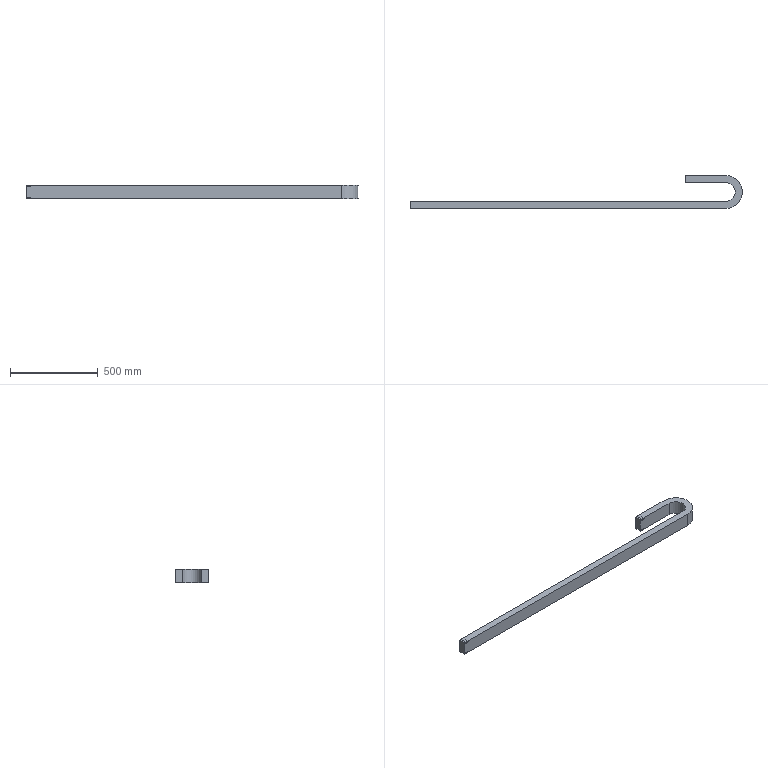Part | SolidWorks | features HoleWzd 2, Extrusion 1 | 1 solid | 26 faces | box 1895 x 190 x 79 mm | volume 7147042 mm3 | cylinder 18 | plane 8 | commonest cylinder face diameters 7 x16 110 x1 190 x1
STEP:
#1=CARTESIAN_POINT('',(-317.901,19.409,1.5));
#2=VERTEX_POINT('',#1);
#3=CARTESIAN_POINT('',(-317.901,19.409,8.5));
#4=VERTEX_POINT('',#3);
#5=CARTESIAN_POINT('',(-317.901,19.409,5.));
#6=DIRECTION('',(0.,1.,0.));
#7=DIRECTION('',(0.,0.,1.));
#8=AXIS2_PLACEMENT_3D('',#5,#6,#7);
#9=CIRCLE('',#8,3.5);
#10=EDGE_CURVE('',#2,#4,#9,.T.);
#11=ORIENTED_EDGE('',*,*,#10,.F.);
#12=CARTESIAN_POINT('',(-317.901,59.409,1.5));
#13=VERTEX_POINT('',#12);
#14=CARTESIAN_POINT('',(-317.901,59.409,1.5));
#15=DIRECTION('',(0.,1.,0.));
#16=VECTOR('',#15,1000.);
#17=LINE('',#14,#16);
#18=EDGE_CURVE('',#2,#13,#17,.T.);
#19=ORIENTED_EDGE('',*,*,#18,.T.);
#20=CARTESIAN_POINT('',(-317.901,59.409,8.5));
#21=VERTEX_POINT('',#20);
#22=CARTESIAN_POINT('',(-317.901,59.409,5.));
#23=DIRECTION('',(0.,1.,0.));
#24=DIRECTION('',(0.,0.,1.));
#25=AXIS2_PLACEMENT_3D('',#22,#23,#24);
#26=CIRCLE('',#25,3.5);
#27=EDGE_CURVE('',#13,#21,#26,.T.);
#28=ORIENTED_EDGE('',*,*,#27,.T.);
#29=CARTESIAN_POINT('',(-317.901,59.409,8.5));
#30=DIRECTION('',(0.,1.,0.));
#31=VECTOR('',#30,1000.);
#32=LINE('',#29,#31);
#33=EDGE_CURVE('',#4,#21,#32,.T.);
#34=ORIENTED_EDGE('',*,*,#33,.F.);
#35=EDGE_LOOP('',(#11,#19,#28,#34));
#36=FACE_OUTER_BOUND('',#35,.T.);
#37=CARTESIAN_POINT('',(-317.901,59.409,5.));
#38=DIRECTION('',(0.,1.,0.));
#39=DIRECTION('',(0.,0.,1.));
#40=AXIS2_PLACEMENT_3D('',#37,#38,#39);
#41=CYLINDRICAL_SURFACE('',#40,3.5);
#42=ADVANCED_FACE('',(#36),#41,.F.);
#43=CARTESIAN_POINT('',(-302.901,19.409,1.5));
#44=VERTEX_POINT('',#43);
#45=CARTESIAN_POINT('',(-302.901,19.409,8.5));
#46=VERTEX_POINT('',#45);
#47=CARTESIAN_POINT('',(-302.901,19.409,5.));
#48=DIRECTION('',(0.,1.,0.));
#49=DIRECTION('',(0.,0.,1.));
#50=AXIS2_PLACEMENT_3D('',#47,#48,#49);
#51=CIRCLE('',#50,3.5);
#52=EDGE_CURVE('',#44,#46,#51,.T.);
#53=ORIENTED_EDGE('',*,*,#52,.F.);
#54=CARTESIAN_POINT('',(-302.901,59.409,1.5));
#55=VERTEX_POINT('',#54);
#56=CARTESIAN_POINT('',(-302.901,59.409,1.5));
#57=DIRECTION('',(0.,1.,0.));
#58=VECTOR('',#57,1000.);
#59=LINE('',#56,#58);
#60=EDGE_CURVE('',#44,#55,#59,.T.);
#61=ORIENTED_EDGE('',*,*,#60,.T.);
#62=CARTESIAN_POINT('',(-302.901,59.409,8.5));
#63=VERTEX_POINT('',#62);
#64=CARTESIAN_POINT('',(-302.901,59.409,5.));
#65=DIRECTION('',(0.,1.,0.));
#66=DIRECTION('',(0.,0.,1.));
#67=AXIS2_PLACEMENT_3D('',#64,#65,#66);
#68=CIRCLE('',#67,3.5);
#69=EDGE_CURVE('',#55,#63,#68,.T.);
#70=ORIENTED_EDGE('',*,*,#69,.T.);
#71=CARTESIAN_POINT('',(-302.901,59.409,8.5));
#72=DIRECTION('',(0.,1.,0.));
#73=VECTOR('',#72,1000.);
#74=LINE('',#71,#73);
#75=EDGE_CURVE('',#46,#63,#74,.T.);
#76=ORIENTED_EDGE('',*,*,#75,.F.);
#77=EDGE_LOOP('',(#53,#61,#70,#76));
#78=FACE_OUTER_BOUND('',#77,.T.);
#79=CARTESIAN_POINT('',(-302.901,59.409,5.));
#80=DIRECTION('',(0.,1.,0.));
#81=DIRECTION('',(0.,0.,1.));
#82=AXIS2_PLACEMENT_3D('',#79,#80,#81);
#83=CYLINDRICAL_SURFACE('',#82,3.5);
#84=ADVANCED_FACE('',(#78),#83,.F.);
#85=CARTESIAN_POINT('',(-317.901,19.409,70.5));
#86=VERTEX_POINT('',#85);
#87=CARTESIAN_POINT('',(-317.901,19.409,77.5));
#88=VERTEX_POINT('',#87);
#89=CARTESIAN_POINT('',(-317.901,19.409,74.));
#90=DIRECTION('',(0.,1.,0.));
#91=DIRECTION('',(0.,0.,1.));
#92=AXIS2_PLACEMENT_3D('',#89,#90,#91);
#93=CIRCLE('',#92,3.5);
#94=EDGE_CURVE('',#86,#88,#93,.T.);
#95=ORIENTED_EDGE('',*,*,#94,.F.);
#96=CARTESIAN_POINT('',(-317.901,59.409,70.5));
#97=VERTEX_POINT('',#96);
#98=CARTESIAN_POINT('',(-317.901,59.409,70.5));
#99=DIRECTION('',(0.,1.,0.));
#100=VECTOR('',#99,1000.);
#101=LINE('',#98,#100);
#102=EDGE_CURVE('',#86,#97,#101,.T.);
#103=ORIENTED_EDGE('',*,*,#102,.T.);
#104=CARTESIAN_POINT('',(-317.901,59.409,77.5));
#105=VERTEX_POINT('',#104);
#106=CARTESIAN_POINT('',(-317.901,59.409,74.));
#107=DIRECTION('',(0.,1.,0.));
#108=DIRECTION('',(0.,0.,1.));
#109=AXIS2_PLACEMENT_3D('',#106,#107,#108);
#110=CIRCLE('',#109,3.5);
#111=EDGE_CURVE('',#97,#105,#110,.T.);
#112=ORIENTED_EDGE('',*,*,#111,.T.);
#113=CARTESIAN_POINT('',(-317.901,59.409,77.5));
#114=DIRECTION('',(0.,1.,0.));
#115=VECTOR('',#114,1000.);
#116=LINE('',#113,#115);
#117=EDGE_CURVE('',#88,#105,#116,.T.);
#118=ORIENTED_EDGE('',*,*,#117,.F.);
#119=EDGE_LOOP('',(#95,#103,#112,#118));
#120=FACE_OUTER_BOUND('',#119,.T.);
#121=CARTESIAN_POINT('',(-317.901,59.409,74.));
#122=DIRECTION('',(0.,1.,0.));
#123=DIRECTION('',(0.,0.,1.));
#124=AXIS2_PLACEMENT_3D('',#121,#122,#123);
#125=CYLINDRICAL_SURFACE('',#124,3.5);
#126=ADVANCED_FACE('',(#120),#125,.F.);
#127=CARTESIAN_POINT('',(-302.901,19.409,70.5));
#128=VERTEX_POINT('',#127);
#129=CARTESIAN_POINT('',(-302.901,19.409,77.5));
#130=VERTEX_POINT('',#129);
#131=CARTESIAN_POINT('',(-302.901,19.409,74.));
#132=DIRECTION('',(0.,1.,0.));
#133=DIRECTION('',(0.,0.,1.));
#134=AXIS2_PLACEMENT_3D('',#131,#132,#133);
#135=CIRCLE('',#134,3.5);
#136=EDGE_CURVE('',#128,#130,#135,.T.);
#137=ORIENTED_EDGE('',*,*,#136,.F.);
#138=CARTESIAN_POINT('',(-302.901,59.409,70.5));
#139=VERTEX_POINT('',#138);
#140=CARTESIAN_POINT('',(-302.901,59.409,70.5));
#141=DIRECTION('',(0.,1.,0.));
#142=VECTOR('',#141,1000.);
#143=LINE('',#140,#142);
#144=EDGE_CURVE('',#128,#139,#143,.T.);
#145=ORIENTED_EDGE('',*,*,#144,.T.);
#146=CARTESIAN_POINT('',(-302.901,59.409,77.5));
#147=VERTEX_POINT('',#146);
#148=CARTESIAN_POINT('',(-302.901,59.409,74.));
#149=DIRECTION('',(0.,1.,0.));
#150=DIRECTION('',(0.,0.,1.));
#151=AXIS2_PLACEMENT_3D('',#148,#149,#150);
#152=CIRCLE('',#151,3.5);
#153=EDGE_CURVE('',#139,#147,#152,.T.);
#154=ORIENTED_EDGE('',*,*,#153,.T.);
#155=CARTESIAN_POINT('',(-302.901,59.409,77.5));
#156=DIRECTION('',(0.,1.,0.));
#157=VECTOR('',#156,1000.);
#158=LINE('',#155,#157);
#159=EDGE_CURVE('',#130,#147,#158,.T.);
#160=ORIENTED_EDGE('',*,*,#159,.F.);
#161=EDGE_LOOP('',(#137,#145,#154,#160));
#162=FACE_OUTER_BOUND('',#161,.T.);
#163=CARTESIAN_POINT('',(-302.901,59.409,74.));
#164=DIRECTION('',(0.,1.,0.));
#165=DIRECTION('',(0.,0.,1.));
#166=AXIS2_PLACEMENT_3D('',#163,#164,#165);
#167=CYLINDRICAL_SURFACE('',#166,3.5);
#168=ADVANCED_FACE('',(#162),#167,.F.);
#169=CARTESIAN_POINT('',(-1872.901,-90.591,8.5));
#170=VERTEX_POINT('',#169);
#171=CARTESIAN_POINT('',(-1872.901,-90.591,1.5));
#172=VERTEX_POINT('',#171);
#173=CARTESIAN_POINT('',(-1872.901,-90.591,5.));
#174=DIRECTION('',(0.,-1.,0.));
#175=DIRECTION('',(1.,0.,0.));
#176=AXIS2_PLACEMENT_3D('',#173,#174,#175);
#177=CIRCLE('',#176,3.5);
#178=EDGE_CURVE('',#170,#172,#177,.T.);
#179=ORIENTED_EDGE('',*,*,#178,.F.);
#180=CARTESIAN_POINT('',(-1872.901,-130.591,8.5));
#181=VERTEX_POINT('',#180);
#182=CARTESIAN_POINT('',(-1872.901,-130.591,8.5));
#183=DIRECTION('',(0.,-1.,0.));
#184=VECTOR('',#183,1000.);
#185=LINE('',#182,#184);
#186=EDGE_CURVE('',#170,#181,#185,.T.);
#187=ORIENTED_EDGE('',*,*,#186,.T.);
#188=CARTESIAN_POINT('',(-1872.901,-130.591,1.5));
#189=VERTEX_POINT('',#188);
#190=CARTESIAN_POINT('',(-1872.901,-130.591,5.));
#191=DIRECTION('',(0.,-1.,0.));
#192=DIRECTION('',(0.,0.,-1.));
#193=AXIS2_PLACEMENT_3D('',#190,#191,#192);
#194=CIRCLE('',#193,3.5);
#195=EDGE_CURVE('',#181,#189,#194,.T.);
#196=ORIENTED_EDGE('',*,*,#195,.T.);
#197=CARTESIAN_POINT('',(-1872.901,-130.591,1.5));
#198=DIRECTION('',(0.,-1.,0.));
#199=VECTOR('',#198,1000.);
#200=LINE('',#197,#199);
#201=EDGE_CURVE('',#172,#189,#200,.T.);
#202=ORIENTED_EDGE('',*,*,#201,.F.);
#203=EDGE_LOOP('',(#179,#187,#196,#202));
#204=FACE_OUTER_BOUND('',#203,.T.);
#205=CARTESIAN_POINT('',(-1872.901,-130.591,5.));
#206=DIRECTION('',(0.,-1.,0.));
#207=DIRECTION('',(0.,0.,-1.));
#208=AXIS2_PLACEMENT_3D('',#205,#206,#207);
#209=CYLINDRICAL_SURFACE('',#208,3.5);
#210=ADVANCED_FACE('',(#204),#209,.F.);
#211=CARTESIAN_POINT('',(-1887.901,-90.591,8.5));
#212=VERTEX_POINT('',#211);
#213=CARTESIAN_POINT('',(-1887.901,-90.591,1.5));
#214=VERTEX_POINT('',#213);
#215=CARTESIAN_POINT('',(-1887.901,-90.591,5.));
#216=DIRECTION('',(0.,-1.,0.));
#217=DIRECTION('',(1.,0.,0.));
#218=AXIS2_PLACEMENT_3D('',#215,#216,#217);
#219=CIRCLE('',#218,3.5);
#220=EDGE_CURVE('',#212,#214,#219,.T.);
#221=ORIENTED_EDGE('',*,*,#220,.F.);
#222=CARTESIAN_POINT('',(-1887.901,-130.591,8.5));
#223=VERTEX_POINT('',#222);
#224=CARTESIAN_POINT('',(-1887.901,-130.591,8.5));
#225=DIRECTION('',(0.,-1.,0.));
#226=VECTOR('',#225,1000.);
#227=LINE('',#224,#226);
#228=EDGE_CURVE('',#212,#223,#227,.T.);
#229=ORIENTED_EDGE('',*,*,#228,.T.);
#230=CARTESIAN_POINT('',(-1887.901,-130.591,1.5));
#231=VERTEX_POINT('',#230);
#232=CARTESIAN_POINT('',(-1887.901,-130.591,5.));
#233=DIRECTION('',(0.,-1.,0.));
#234=DIRECTION('',(0.,0.,-1.));
#235=AXIS2_PLACEMENT_3D('',#232,#233,#234);
#236=CIRCLE('',#235,3.5);
#237=EDGE_CURVE('',#223,#231,#236,.T.);
#238=ORIENTED_EDGE('',*,*,#237,.T.);
#239=CARTESIAN_POINT('',(-1887.901,-130.591,1.5));
#240=DIRECTION('',(0.,-1.,0.));
#241=VECTOR('',#240,1000.);
#242=LINE('',#239,#241);
#243=EDGE_CURVE('',#214,#231,#242,.T.);
#244=ORIENTED_EDGE('',*,*,#243,.F.);
#245=EDGE_LOOP('',(#221,#229,#238,#244));
#246=FACE_OUTER_BOUND('',#245,.T.);
#247=CARTESIAN_POINT('',(-1887.901,-130.591,5.));
#248=DIRECTION('',(0.,-1.,0.));
#249=DIRECTION('',(0.,0.,-1.));
#250=AXIS2_PLACEMENT_3D('',#247,#248,#249);
#251=CYLINDRICAL_SURFACE('',#250,3.5);
#252=ADVANCED_FACE('',(#246),#251,.F.);
#253=CARTESIAN_POINT('',(-1872.901,-90.591,77.5));
#254=VERTEX_POINT('',#253);
#255=CARTESIAN_POINT('',(-1872.901,-90.591,70.5));
#256=VERTEX_POINT('',#255);
#257=CARTESIAN_POINT('',(-1872.901,-90.591,74.));
#258=DIRECTION('',(0.,-1.,0.));
#259=DIRECTION('',(1.,0.,0.));
#260=AXIS2_PLACEMENT_3D('',#257,#258,#259);
#261=CIRCLE('',#260,3.5);
#262=EDGE_CURVE('',#254,#256,#261,.T.);
#263=ORIENTED_EDGE('',*,*,#262,.F.);
#264=CARTESIAN_POINT('',(-1872.901,-130.591,77.5));
#265=VERTEX_POINT('',#264);
#266=CARTESIAN_POINT('',(-1872.901,-130.591,77.5));
#267=DIRECTION('',(0.,-1.,0.));
#268=VECTOR('',#267,1000.);
#269=LINE('',#266,#268);
#270=EDGE_CURVE('',#254,#265,#269,.T.);
#271=ORIENTED_EDGE('',*,*,#270,.T.);
#272=CARTESIAN_POINT('',(-1872.901,-130.591,70.5));
#273=VERTEX_POINT('',#272);
#274=CARTESIAN_POINT('',(-1872.901,-130.591,74.));
#275=DIRECTION('',(0.,-1.,0.));
#276=DIRECTION('',(0.,0.,-1.));
#277=AXIS2_PLACEMENT_3D('',#274,#275,#276);
#278=CIRCLE('',#277,3.5);
#279=EDGE_CURVE('',#265,#273,#278,.T.);
#280=ORIENTED_EDGE('',*,*,#279,.T.);
#281=CARTESIAN_POINT('',(-1872.901,-130.591,70.5));
#282=DIRECTION('',(0.,-1.,0.));
#283=VECTOR('',#282,1000.);
#284=LINE('',#281,#283);
#285=EDGE_CURVE('',#256,#273,#284,.T.);
#286=ORIENTED_EDGE('',*,*,#285,.F.);
#287=EDGE_LOOP('',(#263,#271,#280,#286));
#288=FACE_OUTER_BOUND('',#287,.T.);
#289=CARTESIAN_POINT('',(-1872.901,-130.591,74.));
#290=DIRECTION('',(0.,-1.,0.));
#291=DIRECTION('',(0.,0.,-1.));
#292=AXIS2_PLACEMENT_3D('',#289,#290,#291);
#293=CYLINDRICAL_SURFACE('',#292,3.5);
#294=ADVANCED_FACE('',(#288),#293,.F.);
#295=CARTESIAN_POINT('',(-1887.901,-90.591,77.5));
#296=VERTEX_POINT('',#295);
#297=CARTESIAN_POINT('',(-1887.901,-90.591,70.5));
#298=VERTEX_POINT('',#297);
#299=CARTESIAN_POINT('',(-1887.901,-90.591,74.));
#300=DIRECTION('',(0.,-1.,0.));
#301=DIRECTION('',(1.,0.,0.));
#302=AXIS2_PLACEMENT_3D('',#299,#300,#301);
#303=CIRCLE('',#302,3.5);
#304=EDGE_CURVE('',#296,#298,#303,.T.);
#305=ORIENTED_EDGE('',*,*,#304,.F.);
#306=CARTESIAN_POINT('',(-1887.901,-130.591,77.5));
#307=VERTEX_POINT('',#306);
#308=CARTESIAN_POINT('',(-1887.901,-130.591,77.5));
#309=DIRECTION('',(0.,-1.,0.));
#310=VECTOR('',#309,1000.);
#311=LINE('',#308,#310);
#312=EDGE_CURVE('',#296,#307,#311,.T.);
#313=ORIENTED_EDGE('',*,*,#312,.T.);
#314=CARTESIAN_POINT('',(-1887.901,-130.591,70.5));
#315=VERTEX_POINT('',#314);
#316=CARTESIAN_POINT('',(-1887.901,-130.591,74.));
#317=DIRECTION('',(0.,-1.,0.));
#318=DIRECTION('',(0.,0.,-1.));
#319=AXIS2_PLACEMENT_3D('',#316,#317,#318);
#320=CIRCLE('',#319,3.5);
#321=EDGE_CURVE('',#307,#315,#320,.T.);
#322=ORIENTED_EDGE('',*,*,#321,.T.);
#323=CARTESIAN_POINT('',(-1887.901,-130.591,70.5));
#324=DIRECTION('',(0.,-1.,0.));
#325=VECTOR('',#324,1000.);
#326=LINE('',#323,#325);
#327=EDGE_CURVE('',#298,#315,#326,.T.);
#328=ORIENTED_EDGE('',*,*,#327,.F.);
#329=EDGE_LOOP('',(#305,#313,#322,#328));
#330=FACE_OUTER_BOUND('',#329,.T.);
#331=CARTESIAN_POINT('',(-1887.901,-130.591,74.));
#332=DIRECTION('',(0.,-1.,0.));
#333=DIRECTION('',(0.,0.,-1.));
#334=AXIS2_PLACEMENT_3D('',#331,#332,#333);
#335=CYLINDRICAL_SURFACE('',#334,3.5);
#336=ADVANCED_FACE('',(#330),#335,.F.);
#337=CARTESIAN_POINT('',(-1872.901,-130.591,5.));
#338=DIRECTION('',(0.,-1.,0.));
#339=DIRECTION('',(0.,0.,-1.));
#340=AXIS2_PLACEMENT_3D('',#337,#338,#339);
#341=CIRCLE('',#340,3.5);
#342=EDGE_CURVE('',#189,#181,#341,.T.);
#343=ORIENTED_EDGE('',*,*,#342,.F.);
#344=ORIENTED_EDGE('',*,*,#195,.F.);
#345=EDGE_LOOP('',(#343,#344));
#346=FACE_BOUND('',#345,.T.);
#347=CARTESIAN_POINT('',(-1887.901,-130.591,5.));
#348=DIRECTION('',(0.,-1.,0.));
#349=DIRECTION('',(0.,0.,-1.));
#350=AXIS2_PLACEMENT_3D('',#347,#348,#349);
#351=CIRCLE('',#350,3.5);
#352=EDGE_CURVE('',#231,#223,#351,.T.);
#353=ORIENTED_EDGE('',*,*,#352,.F.);
#354=ORIENTED_EDGE('',*,*,#237,.F.);
#355=EDGE_LOOP('',(#353,#354));
#356=FACE_BOUND('',#355,.T.);
#357=CARTESIAN_POINT('',(-1872.901,-130.591,74.));
#358=DIRECTION('',(0.,-1.,0.));
#359=DIRECTION('',(0.,0.,-1.));
#360=AXIS2_PLACEMENT_3D('',#357,#358,#359);
#361=CIRCLE('',#360,3.5);
#362=EDGE_CURVE('',#273,#265,#361,.T.);
#363=ORIENTED_EDGE('',*,*,#362,.F.);
#364=ORIENTED_EDGE('',*,*,#279,.F.);
#365=EDGE_LOOP('',(#363,#364));
#366=FACE_BOUND('',#365,.T.);
#367=CARTESIAN_POINT('',(-1887.901,-130.591,74.));
#368=DIRECTION('',(0.,-1.,0.));
#369=DIRECTION('',(0.,0.,-1.));
#370=AXIS2_PLACEMENT_3D('',#367,#368,#369);
#371=CIRCLE('',#370,3.5);
#372=EDGE_CURVE('',#315,#307,#371,.T.);
#373=ORIENTED_EDGE('',*,*,#372,.F.);
#374=ORIENTED_EDGE('',*,*,#321,.F.);
#375=EDGE_LOOP('',(#373,#374));
#376=FACE_BOUND('',#375,.T.);
#377=CARTESIAN_POINT('',(-97.901,-130.591,0.));
#378=VERTEX_POINT('',#377);
#379=CARTESIAN_POINT('',(-1897.901,-130.591,0.));
#380=VERTEX_POINT('',#379);
#381=CARTESIAN_POINT('',(0.,-130.591,0.));
#382=DIRECTION('',(-1.,0.,0.));
#383=VECTOR('',#382,1000.);
#384=LINE('',#381,#383);
#385=EDGE_CURVE('',#378,#380,#384,.T.);
#386=ORIENTED_EDGE('',*,*,#385,.F.);
#387=CARTESIAN_POINT('',(-97.901,-130.591,79.));
#388=VERTEX_POINT('',#387);
#389=CARTESIAN_POINT('',(-97.901,-130.591,79.));
#390=DIRECTION('',(0.,0.,-1.));
#391=VECTOR('',#390,1000.);
#392=LINE('',#389,#391);
#393=EDGE_CURVE('',#388,#378,#392,.T.);
#394=ORIENTED_EDGE('',*,*,#393,.F.);
#395=CARTESIAN_POINT('',(-1897.901,-130.591,79.));
#396=VERTEX_POINT('',#395);
#397=CARTESIAN_POINT('',(0.,-130.591,79.));
#398=DIRECTION('',(-1.,0.,0.));
#399=VECTOR('',#398,1000.);
#400=LINE('',#397,#399);
#401=EDGE_CURVE('',#388,#396,#400,.T.);
#402=ORIENTED_EDGE('',*,*,#401,.T.);
#403=CARTESIAN_POINT('',(-1897.901,-130.591,79.));
#404=DIRECTION('',(0.,0.,-1.));
#405=VECTOR('',#404,1000.);
#406=LINE('',#403,#405);
#407=EDGE_CURVE('',#396,#380,#406,.T.);
#408=ORIENTED_EDGE('',*,*,#407,.T.);
#409=EDGE_LOOP('',(#386,#394,#402,#408));
#410=FACE_OUTER_BOUND('',#409,.T.);
#411=CARTESIAN_POINT('',(0.,-130.591,79.));
#412=DIRECTION('',(0.,-1.,0.));
#413=DIRECTION('',(1.,0.,0.));
#414=AXIS2_PLACEMENT_3D('',#411,#412,#413);
#415=PLANE('',#414);
#416=ADVANCED_FACE('',(#346,#356,#366,#376,#410),#415,.T.);
#417=CARTESIAN_POINT('',(-97.901,59.409,0.));
#418=VERTEX_POINT('',#417);
#419=CARTESIAN_POINT('',(-97.901,-35.591,0.));
#420=DIRECTION('',(0.,0.,1.));
#421=DIRECTION('',(1.,0.,0.));
#422=AXIS2_PLACEMENT_3D('',#419,#420,#421);
#423=CIRCLE('',#422,95.);
#424=EDGE_CURVE('',#378,#418,#423,.T.);
#425=ORIENTED_EDGE('',*,*,#424,.T.);
#426=CARTESIAN_POINT('',(-97.901,59.409,79.));
#427=VERTEX_POINT('',#426);
#428=CARTESIAN_POINT('',(-97.901,59.409,79.));
#429=DIRECTION('',(0.,0.,-1.));
#430=VECTOR('',#429,1000.);
#431=LINE('',#428,#430);
#432=EDGE_CURVE('',#427,#418,#431,.T.);
#433=ORIENTED_EDGE('',*,*,#432,.F.);
#434=CARTESIAN_POINT('',(-97.901,-35.591,79.));
#435=DIRECTION('',(0.,0.,1.));
#436=DIRECTION('',(1.,0.,0.));
#437=AXIS2_PLACEMENT_3D('',#434,#435,#436);
#438=CIRCLE('',#437,95.);
#439=EDGE_CURVE('',#388,#427,#438,.T.);
#440=ORIENTED_EDGE('',*,*,#439,.F.);
#441=ORIENTED_EDGE('',*,*,#393,.T.);
#442=EDGE_LOOP('',(#425,#433,#440,#441));
#443=FACE_OUTER_BOUND('',#442,.T.);
#444=CARTESIAN_POINT('',(-97.901,-35.591,79.));
#445=DIRECTION('',(0.,0.,-1.));
#446=DIRECTION('',(-1.,0.,0.));
#447=AXIS2_PLACEMENT_3D('',#444,#445,#446);
#448=CYLINDRICAL_SURFACE('',#447,95.);
#449=ADVANCED_FACE('',(#443),#448,.T.);
#450=CARTESIAN_POINT('',(-317.901,59.409,5.));
#451=DIRECTION('',(0.,1.,0.));
#452=DIRECTION('',(0.,0.,1.));
#453=AXIS2_PLACEMENT_3D('',#450,#451,#452);
#454=CIRCLE('',#453,3.5);
#455=EDGE_CURVE('',#21,#13,#454,.T.);
#456=ORIENTED_EDGE('',*,*,#455,.F.);
#457=ORIENTED_EDGE('',*,*,#27,.F.);
#458=EDGE_LOOP('',(#456,#457));
#459=FACE_BOUND('',#458,.T.);
#460=CARTESIAN_POINT('',(-302.901,59.409,5.));
#461=DIRECTION('',(0.,1.,0.));
#462=DIRECTION('',(0.,0.,1.));
#463=AXIS2_PLACEMENT_3D('',#460,#461,#462);
#464=CIRCLE('',#463,3.5);
#465=EDGE_CURVE('',#63,#55,#464,.T.);
#466=ORIENTED_EDGE('',*,*,#465,.F.);
#467=ORIENTED_EDGE('',*,*,#69,.F.);
#468=EDGE_LOOP('',(#466,#467));
#469=FACE_BOUND('',#468,.T.);
#470=CARTESIAN_POINT('',(-317.901,59.409,74.));
#471=DIRECTION('',(0.,1.,0.));
#472=DIRECTION('',(0.,0.,1.));
#473=AXIS2_PLACEMENT_3D('',#470,#471,#472);
#474=CIRCLE('',#473,3.5);
#475=EDGE_CURVE('',#105,#97,#474,.T.);
#476=ORIENTED_EDGE('',*,*,#475,.F.);
#477=ORIENTED_EDGE('',*,*,#111,.F.);
#478=EDGE_LOOP('',(#476,#477));
#479=FACE_BOUND('',#478,.T.);
#480=CARTESIAN_POINT('',(-302.901,59.409,74.));
#481=DIRECTION('',(0.,1.,0.));
#482=DIRECTION('',(0.,0.,1.));
#483=AXIS2_PLACEMENT_3D('',#480,#481,#482);
#484=CIRCLE('',#483,3.5);
#485=EDGE_CURVE('',#147,#139,#484,.T.);
#486=ORIENTED_EDGE('',*,*,#485,.F.);
#487=ORIENTED_EDGE('',*,*,#153,.F.);
#488=EDGE_LOOP('',(#486,#487));
#489=FACE_BOUND('',#488,.T.);
#490=CARTESIAN_POINT('',(-327.901,59.409,0.));
#491=VERTEX_POINT('',#490);
#492=CARTESIAN_POINT('',(0.,59.409,0.));
#493=DIRECTION('',(1.,0.,0.));
#494=VECTOR('',#493,1000.);
#495=LINE('',#492,#494);
#496=EDGE_CURVE('',#491,#418,#495,.T.);
#497=ORIENTED_EDGE('',*,*,#496,.F.);
#498=CARTESIAN_POINT('',(-327.901,59.409,79.));
#499=VERTEX_POINT('',#498);
#500=CARTESIAN_POINT('',(-327.901,59.409,79.));
#501=DIRECTION('',(0.,0.,-1.));
#502=VECTOR('',#501,1000.);
#503=LINE('',#500,#502);
#504=EDGE_CURVE('',#499,#491,#503,.T.);
#505=ORIENTED_EDGE('',*,*,#504,.F.);
#506=CARTESIAN_POINT('',(0.,59.409,79.));
#507=DIRECTION('',(1.,0.,0.));
#508=VECTOR('',#507,1000.);
#509=LINE('',#506,#508);
#510=EDGE_CURVE('',#499,#427,#509,.T.);
#511=ORIENTED_EDGE('',*,*,#510,.T.);
#512=ORIENTED_EDGE('',*,*,#432,.T.);
#513=EDGE_LOOP('',(#497,#505,#511,#512));
#514=FACE_OUTER_BOUND('',#513,.T.);
#515=CARTESIAN_POINT('',(0.,59.409,79.));
#516=DIRECTION('',(0.,1.,0.));
#517=DIRECTION('',(0.,0.,1.));
#518=AXIS2_PLACEMENT_3D('',#515,#516,#517);
#519=PLANE('',#518);
#520=ADVANCED_FACE('',(#459,#469,#479,#489,#514),#519,.T.);
#521=CARTESIAN_POINT('',(-327.901,19.409,0.));
#522=VERTEX_POINT('',#521);
#523=CARTESIAN_POINT('',(-327.901,0.,0.));
#524=DIRECTION('',(0.,-1.,0.));
#525=VECTOR('',#524,1000.);
#526=LINE('',#523,#525);
#527=EDGE_CURVE('',#491,#522,#526,.T.);
#528=ORIENTED_EDGE('',*,*,#527,.T.);
#529=CARTESIAN_POINT('',(-327.901,19.409,79.));
#530=VERTEX_POINT('',#529);
#531=CARTESIAN_POINT('',(-327.901,19.409,79.));
#532=DIRECTION('',(0.,0.,-1.));
#533=VECTOR('',#532,1000.);
#534=LINE('',#531,#533);
#535=EDGE_CURVE('',#530,#522,#534,.T.);
#536=ORIENTED_EDGE('',*,*,#535,.F.);
#537=CARTESIAN_POINT('',(-327.901,0.,79.));
#538=DIRECTION('',(0.,-1.,0.));
#539=VECTOR('',#538,1000.);
#540=LINE('',#537,#539);
#541=EDGE_CURVE('',#499,#530,#540,.T.);
#542=ORIENTED_EDGE('',*,*,#541,.F.);
#543=ORIENTED_EDGE('',*,*,#504,.T.);
#544=EDGE_LOOP('',(#528,#536,#542,#543));
#545=FACE_OUTER_BOUND('',#544,.T.);
#546=CARTESIAN_POINT('',(-327.901,0.,79.));
#547=DIRECTION('',(1.,0.,0.));
#548=DIRECTION('',(0.,0.,-1.));
#549=AXIS2_PLACEMENT_3D('',#546,#547,#548);
#550=PLANE('',#549);
#551=ADVANCED_FACE('',(#545),#550,.F.);
#552=CARTESIAN_POINT('',(-317.901,19.409,5.));
#553=DIRECTION('',(0.,1.,0.));
#554=DIRECTION('',(0.,0.,1.));
#555=AXIS2_PLACEMENT_3D('',#552,#553,#554);
#556=CIRCLE('',#555,3.5);
#557=EDGE_CURVE('',#4,#2,#556,.T.);
#558=ORIENTED_EDGE('',*,*,#557,.T.);
#559=ORIENTED_EDGE('',*,*,#10,.T.);
#560=EDGE_LOOP('',(#558,#559));
#561=FACE_BOUND('',#560,.T.);
#562=CARTESIAN_POINT('',(-302.901,19.409,5.));
#563=DIRECTION('',(0.,1.,0.));
#564=DIRECTION('',(0.,0.,1.));
#565=AXIS2_PLACEMENT_3D('',#562,#563,#564);
#566=CIRCLE('',#565,3.5);
#567=EDGE_CURVE('',#46,#44,#566,.T.);
#568=ORIENTED_EDGE('',*,*,#567,.T.);
#569=ORIENTED_EDGE('',*,*,#52,.T.);
#570=EDGE_LOOP('',(#568,#569));
#571=FACE_BOUND('',#570,.T.);
#572=CARTESIAN_POINT('',(-317.901,19.409,74.));
#573=DIRECTION('',(0.,1.,0.));
#574=DIRECTION('',(0.,0.,1.));
#575=AXIS2_PLACEMENT_3D('',#572,#573,#574);
#576=CIRCLE('',#575,3.5);
#577=EDGE_CURVE('',#88,#86,#576,.T.);
#578=ORIENTED_EDGE('',*,*,#577,.T.);
#579=ORIENTED_EDGE('',*,*,#94,.T.);
#580=EDGE_LOOP('',(#578,#579));
#581=FACE_BOUND('',#580,.T.);
#582=CARTESIAN_POINT('',(-302.901,19.409,74.));
#583=DIRECTION('',(0.,1.,0.));
#584=DIRECTION('',(0.,0.,1.));
#585=AXIS2_PLACEMENT_3D('',#582,#583,#584);
#586=CIRCLE('',#585,3.5);
#587=EDGE_CURVE('',#130,#128,#586,.T.);
#588=ORIENTED_EDGE('',*,*,#587,.T.);
#589=ORIENTED_EDGE('',*,*,#136,.T.);
#590=EDGE_LOOP('',(#588,#589));
#591=FACE_BOUND('',#590,.T.);
#592=CARTESIAN_POINT('',(-97.901,19.409,0.));
#593=VERTEX_POINT('',#592);
#594=CARTESIAN_POINT('',(0.,19.409,0.));
#595=DIRECTION('',(1.,0.,0.));
#596=VECTOR('',#595,1000.);
#597=LINE('',#594,#596);
#598=EDGE_CURVE('',#522,#593,#597,.T.);
#599=ORIENTED_EDGE('',*,*,#598,.T.);
#600=CARTESIAN_POINT('',(-97.901,19.409,79.));
#601=VERTEX_POINT('',#600);
#602=CARTESIAN_POINT('',(-97.901,19.409,79.));
#603=DIRECTION('',(0.,0.,-1.));
#604=VECTOR('',#603,1000.);
#605=LINE('',#602,#604);
#606=EDGE_CURVE('',#601,#593,#605,.T.);
#607=ORIENTED_EDGE('',*,*,#606,.F.);
#608=CARTESIAN_POINT('',(0.,19.409,79.));
#609=DIRECTION('',(1.,0.,0.));
#610=VECTOR('',#609,1000.);
#611=LINE('',#608,#610);
#612=EDGE_CURVE('',#530,#601,#611,.T.);
#613=ORIENTED_EDGE('',*,*,#612,.F.);
#614=ORIENTED_EDGE('',*,*,#535,.T.);
#615=EDGE_LOOP('',(#599,#607,#613,#614));
#616=FACE_OUTER_BOUND('',#615,.T.);
#617=CARTESIAN_POINT('',(0.,19.409,79.));
#618=DIRECTION('',(0.,1.,0.));
#619=DIRECTION('',(0.,0.,1.));
#620=AXIS2_PLACEMENT_3D('',#617,#618,#619);
#621=PLANE('',#620);
#622=ADVANCED_FACE('',(#561,#571,#581,#591,#616),#621,.F.);
#623=CARTESIAN_POINT('',(-97.901,-90.591,0.));
#624=VERTEX_POINT('',#623);
#625=CARTESIAN_POINT('',(-97.901,-35.591,0.));
#626=DIRECTION('',(0.,0.,1.));
#627=DIRECTION('',(1.,0.,0.));
#628=AXIS2_PLACEMENT_3D('',#625,#626,#627);
#629=CIRCLE('',#628,55.);
#630=EDGE_CURVE('',#624,#593,#629,.T.);
#631=ORIENTED_EDGE('',*,*,#630,.F.);
#632=CARTESIAN_POINT('',(-97.901,-90.591,79.));
#633=VERTEX_POINT('',#632);
#634=CARTESIAN_POINT('',(-97.901,-90.591,79.));
#635=DIRECTION('',(0.,0.,-1.));
#636=VECTOR('',#635,1000.);
#637=LINE('',#634,#636);
#638=EDGE_CURVE('',#633,#624,#637,.T.);
#639=ORIENTED_EDGE('',*,*,#638,.F.);
#640=CARTESIAN_POINT('',(-97.901,-35.591,79.));
#641=DIRECTION('',(0.,0.,1.));
#642=DIRECTION('',(1.,0.,0.));
#643=AXIS2_PLACEMENT_3D('',#640,#641,#642);
#644=CIRCLE('',#643,55.);
#645=EDGE_CURVE('',#633,#601,#644,.T.);
#646=ORIENTED_EDGE('',*,*,#645,.T.);
#647=ORIENTED_EDGE('',*,*,#606,.T.);
#648=EDGE_LOOP('',(#631,#639,#646,#647));
#649=FACE_OUTER_BOUND('',#648,.T.);
#650=CARTESIAN_POINT('',(-97.901,-35.591,79.));
#651=DIRECTION('',(0.,0.,-1.));
#652=DIRECTION('',(-1.,0.,0.));
#653=AXIS2_PLACEMENT_3D('',#650,#651,#652);
#654=CYLINDRICAL_SURFACE('',#653,55.);
#655=ADVANCED_FACE('',(#649),#654,.F.);
#656=CARTESIAN_POINT('',(-1872.901,-90.591,5.));
#657=DIRECTION('',(0.,-1.,0.));
#658=DIRECTION('',(1.,0.,0.));
#659=AXIS2_PLACEMENT_3D('',#656,#657,#658);
#660=CIRCLE('',#659,3.5);
#661=EDGE_CURVE('',#172,#170,#660,.T.);
#662=ORIENTED_EDGE('',*,*,#661,.T.);
#663=ORIENTED_EDGE('',*,*,#178,.T.);
#664=EDGE_LOOP('',(#662,#663));
#665=FACE_BOUND('',#664,.T.);
#666=CARTESIAN_POINT('',(-1887.901,-90.591,5.));
#667=DIRECTION('',(0.,-1.,0.));
#668=DIRECTION('',(1.,0.,0.));
#669=AXIS2_PLACEMENT_3D('',#666,#667,#668);
#670=CIRCLE('',#669,3.5);
#671=EDGE_CURVE('',#214,#212,#670,.T.);
#672=ORIENTED_EDGE('',*,*,#671,.T.);
#673=ORIENTED_EDGE('',*,*,#220,.T.);
#674=EDGE_LOOP('',(#672,#673));
#675=FACE_BOUND('',#674,.T.);
#676=CARTESIAN_POINT('',(-1872.901,-90.591,74.));
#677=DIRECTION('',(0.,-1.,0.));
#678=DIRECTION('',(1.,0.,0.));
#679=AXIS2_PLACEMENT_3D('',#676,#677,#678);
#680=CIRCLE('',#679,3.5);
#681=EDGE_CURVE('',#256,#254,#680,.T.);
#682=ORIENTED_EDGE('',*,*,#681,.T.);
#683=ORIENTED_EDGE('',*,*,#262,.T.);
#684=EDGE_LOOP('',(#682,#683));
#685=FACE_BOUND('',#684,.T.);
#686=CARTESIAN_POINT('',(-1887.901,-90.591,74.));
#687=DIRECTION('',(0.,-1.,0.));
#688=DIRECTION('',(1.,0.,0.));
#689=AXIS2_PLACEMENT_3D('',#686,#687,#688);
#690=CIRCLE('',#689,3.5);
#691=EDGE_CURVE('',#298,#296,#690,.T.);
#692=ORIENTED_EDGE('',*,*,#691,.T.);
#693=ORIENTED_EDGE('',*,*,#304,.T.);
#694=EDGE_LOOP('',(#692,#693));
#695=FACE_BOUND('',#694,.T.);
#696=CARTESIAN_POINT('',(-1897.901,-90.591,0.));
#697=VERTEX_POINT('',#696);
#698=CARTESIAN_POINT('',(0.,-90.591,0.));
#699=DIRECTION('',(-1.,0.,0.));
#700=VECTOR('',#699,1000.);
#701=LINE('',#698,#700);
#702=EDGE_CURVE('',#624,#697,#701,.T.);
#703=ORIENTED_EDGE('',*,*,#702,.T.);
#704=CARTESIAN_POINT('',(-1897.901,-90.591,79.));
#705=VERTEX_POINT('',#704);
#706=CARTESIAN_POINT('',(-1897.901,-90.591,79.));
#707=DIRECTION('',(0.,0.,-1.));
#708=VECTOR('',#707,1000.);
#709=LINE('',#706,#708);
#710=EDGE_CURVE('',#705,#697,#709,.T.);
#711=ORIENTED_EDGE('',*,*,#710,.F.);
#712=CARTESIAN_POINT('',(0.,-90.591,79.));
#713=DIRECTION('',(-1.,0.,0.));
#714=VECTOR('',#713,1000.);
#715=LINE('',#712,#714);
#716=EDGE_CURVE('',#633,#705,#715,.T.);
#717=ORIENTED_EDGE('',*,*,#716,.F.);
#718=ORIENTED_EDGE('',*,*,#638,.T.);
#719=EDGE_LOOP('',(#703,#711,#717,#718));
#720=FACE_OUTER_BOUND('',#719,.T.);
#721=CARTESIAN_POINT('',(0.,-90.591,79.));
#722=DIRECTION('',(0.,-1.,0.));
#723=DIRECTION('',(1.,0.,0.));
#724=AXIS2_PLACEMENT_3D('',#721,#722,#723);
#725=PLANE('',#724);
#726=ADVANCED_FACE('',(#665,#675,#685,#695,#720),#725,.F.);
#727=CARTESIAN_POINT('',(-1897.901,0.,0.));
#728=DIRECTION('',(0.,-1.,0.));
#729=VECTOR('',#728,1000.);
#730=LINE('',#727,#729);
#731=EDGE_CURVE('',#697,#380,#730,.T.);
#732=ORIENTED_EDGE('',*,*,#731,.T.);
#733=ORIENTED_EDGE('',*,*,#407,.F.);
#734=CARTESIAN_POINT('',(-1897.901,0.,79.));
#735=DIRECTION('',(0.,-1.,0.));
#736=VECTOR('',#735,1000.);
#737=LINE('',#734,#736);
#738=EDGE_CURVE('',#705,#396,#737,.T.);
#739=ORIENTED_EDGE('',*,*,#738,.F.);
#740=ORIENTED_EDGE('',*,*,#710,.T.);
#741=EDGE_LOOP('',(#732,#733,#739,#740));
#742=FACE_OUTER_BOUND('',#741,.T.);
#743=CARTESIAN_POINT('',(-1897.901,0.,79.));
#744=DIRECTION('',(1.,0.,0.));
#745=DIRECTION('',(0.,0.,-1.));
#746=AXIS2_PLACEMENT_3D('',#743,#744,#745);
#747=PLANE('',#746);
#748=ADVANCED_FACE('',(#742),#747,.F.);
#749=ORIENTED_EDGE('',*,*,#401,.F.);
#750=ORIENTED_EDGE('',*,*,#439,.T.);
#751=ORIENTED_EDGE('',*,*,#510,.F.);
#752=ORIENTED_EDGE('',*,*,#541,.T.);
#753=ORIENTED_EDGE('',*,*,#612,.T.);
#754=ORIENTED_EDGE('',*,*,#645,.F.);
#755=ORIENTED_EDGE('',*,*,#716,.T.);
#756=ORIENTED_EDGE('',*,*,#738,.T.);
#757=EDGE_LOOP('',(#749,#750,#751,#752,#753,#754,#755,#756));
#758=FACE_OUTER_BOUND('',#757,.T.);
#759=CARTESIAN_POINT('',(0.,0.,79.));
#760=DIRECTION('',(0.,0.,1.));
#761=DIRECTION('',(1.,0.,0.));
#762=AXIS2_PLACEMENT_3D('',#759,#760,#761);
#763=PLANE('',#762);
#764=ADVANCED_FACE('',(#758),#763,.T.);
#765=ORIENTED_EDGE('',*,*,#385,.T.);
#766=ORIENTED_EDGE('',*,*,#731,.F.);
#767=ORIENTED_EDGE('',*,*,#702,.F.);
#768=ORIENTED_EDGE('',*,*,#630,.T.);
#769=ORIENTED_EDGE('',*,*,#598,.F.);
#770=ORIENTED_EDGE('',*,*,#527,.F.);
#771=ORIENTED_EDGE('',*,*,#496,.T.);
#772=ORIENTED_EDGE('',*,*,#424,.F.);
#773=EDGE_LOOP('',(#765,#766,#767,#768,#769,#770,#771,#772));
#774=FACE_OUTER_BOUND('',#773,.T.);
#775=CARTESIAN_POINT('',(0.,0.,0.));
#776=DIRECTION('',(0.,0.,1.));
#777=DIRECTION('',(1.,0.,0.));
#778=AXIS2_PLACEMENT_3D('',#775,#776,#777);
#779=PLANE('',#778);
#780=ADVANCED_FACE('',(#774),#779,.F.);
#781=ORIENTED_EDGE('',*,*,#312,.F.);
#782=ORIENTED_EDGE('',*,*,#691,.F.);
#783=ORIENTED_EDGE('',*,*,#327,.T.);
#784=ORIENTED_EDGE('',*,*,#372,.T.);
#785=EDGE_LOOP('',(#781,#782,#783,#784));
#786=FACE_OUTER_BOUND('',#785,.T.);
#787=CARTESIAN_POINT('',(-1887.901,-130.591,74.));
#788=DIRECTION('',(0.,-1.,0.));
#789=DIRECTION('',(0.,0.,-1.));
#790=AXIS2_PLACEMENT_3D('',#787,#788,#789);
#791=CYLINDRICAL_SURFACE('',#790,3.5);
#792=ADVANCED_FACE('',(#786),#791,.F.);
#793=ORIENTED_EDGE('',*,*,#270,.F.);
#794=ORIENTED_EDGE('',*,*,#681,.F.);
#795=ORIENTED_EDGE('',*,*,#285,.T.);
#796=ORIENTED_EDGE('',*,*,#362,.T.);
#797=EDGE_LOOP('',(#793,#794,#795,#796));
#798=FACE_OUTER_BOUND('',#797,.T.);
#799=CARTESIAN_POINT('',(-1872.901,-130.591,74.));
#800=DIRECTION('',(0.,-1.,0.));
#801=DIRECTION('',(0.,0.,-1.));
#802=AXIS2_PLACEMENT_3D('',#799,#800,#801);
#803=CYLINDRICAL_SURFACE('',#802,3.5);
#804=ADVANCED_FACE('',(#798),#803,.F.);
#805=ORIENTED_EDGE('',*,*,#228,.F.);
#806=ORIENTED_EDGE('',*,*,#671,.F.);
#807=ORIENTED_EDGE('',*,*,#243,.T.);
#808=ORIENTED_EDGE('',*,*,#352,.T.);
#809=EDGE_LOOP('',(#805,#806,#807,#808));
#810=FACE_OUTER_BOUND('',#809,.T.);
#811=CARTESIAN_POINT('',(-1887.901,-130.591,5.));
#812=DIRECTION('',(0.,-1.,0.));
#813=DIRECTION('',(0.,0.,-1.));
#814=AXIS2_PLACEMENT_3D('',#811,#812,#813);
#815=CYLINDRICAL_SURFACE('',#814,3.5);
#816=ADVANCED_FACE('',(#810),#815,.F.);
#817=ORIENTED_EDGE('',*,*,#186,.F.);
#818=ORIENTED_EDGE('',*,*,#661,.F.);
#819=ORIENTED_EDGE('',*,*,#201,.T.);
#820=ORIENTED_EDGE('',*,*,#342,.T.);
#821=EDGE_LOOP('',(#817,#818,#819,#820));
#822=FACE_OUTER_BOUND('',#821,.T.);
#823=CARTESIAN_POINT('',(-1872.901,-130.591,5.));
#824=DIRECTION('',(0.,-1.,0.));
#825=DIRECTION('',(0.,0.,-1.));
#826=AXIS2_PLACEMENT_3D('',#823,#824,#825);
#827=CYLINDRICAL_SURFACE('',#826,3.5);
#828=ADVANCED_FACE('',(#822),#827,.F.);
#829=ORIENTED_EDGE('',*,*,#144,.F.);
#830=ORIENTED_EDGE('',*,*,#587,.F.);
#831=ORIENTED_EDGE('',*,*,#159,.T.);
#832=ORIENTED_EDGE('',*,*,#485,.T.);
#833=EDGE_LOOP('',(#829,#830,#831,#832));
#834=FACE_OUTER_BOUND('',#833,.T.);
#835=CARTESIAN_POINT('',(-302.901,59.409,74.));
#836=DIRECTION('',(0.,1.,0.));
#837=DIRECTION('',(0.,0.,1.));
#838=AXIS2_PLACEMENT_3D('',#835,#836,#837);
#839=CYLINDRICAL_SURFACE('',#838,3.5);
#840=ADVANCED_FACE('',(#834),#839,.F.);
#841=ORIENTED_EDGE('',*,*,#102,.F.);
#842=ORIENTED_EDGE('',*,*,#577,.F.);
#843=ORIENTED_EDGE('',*,*,#117,.T.);
#844=ORIENTED_EDGE('',*,*,#475,.T.);
#845=EDGE_LOOP('',(#841,#842,#843,#844));
#846=FACE_OUTER_BOUND('',#845,.T.);
#847=CARTESIAN_POINT('',(-317.901,59.409,74.));
#848=DIRECTION('',(0.,1.,0.));
#849=DIRECTION('',(0.,0.,1.));
#850=AXIS2_PLACEMENT_3D('',#847,#848,#849);
#851=CYLINDRICAL_SURFACE('',#850,3.5);
#852=ADVANCED_FACE('',(#846),#851,.F.);
#853=ORIENTED_EDGE('',*,*,#60,.F.);
#854=ORIENTED_EDGE('',*,*,#567,.F.);
#855=ORIENTED_EDGE('',*,*,#75,.T.);
#856=ORIENTED_EDGE('',*,*,#465,.T.);
#857=EDGE_LOOP('',(#853,#854,#855,#856));
#858=FACE_OUTER_BOUND('',#857,.T.);
#859=CARTESIAN_POINT('',(-302.901,59.409,5.));
#860=DIRECTION('',(0.,1.,0.));
#861=DIRECTION('',(0.,0.,1.));
#862=AXIS2_PLACEMENT_3D('',#859,#860,#861);
#863=CYLINDRICAL_SURFACE('',#862,3.5);
#864=ADVANCED_FACE('',(#858),#863,.F.);
#865=ORIENTED_EDGE('',*,*,#18,.F.);
#866=ORIENTED_EDGE('',*,*,#557,.F.);
#867=ORIENTED_EDGE('',*,*,#33,.T.);
#868=ORIENTED_EDGE('',*,*,#455,.T.);
#869=EDGE_LOOP('',(#865,#866,#867,#868));
#870=FACE_OUTER_BOUND('',#869,.T.);
#871=CARTESIAN_POINT('',(-317.901,59.409,5.));
#872=DIRECTION('',(0.,1.,0.));
#873=DIRECTION('',(0.,0.,1.));
#874=AXIS2_PLACEMENT_3D('',#871,#872,#873);
#875=CYLINDRICAL_SURFACE('',#874,3.5);
#876=ADVANCED_FACE('',(#870),#875,.F.);
#877=CLOSED_SHELL('',(#42,#84,#126,#168,#210,#252,#294,#336,#416,#449,#520,#551,#622,#655,#726,#748,#764,#780,#792,#804,#816,#828,#840,#852,#864,#876));
#878=MANIFOLD_SOLID_BREP('',#877);
#879=CARTESIAN_POINT('',(0.,0.,0.));
#880=DIRECTION('',(0.,0.,1.));
#881=DIRECTION('',(1.,0.,0.));
#882=AXIS2_PLACEMENT_3D('',#879,#880,#881);
#883=(LENGTH_UNIT()NAMED_UNIT(*)SI_UNIT(.MILLI.,.METRE.));
#884=UNCERTAINTY_MEASURE_WITH_UNIT(LENGTH_MEASURE(0.00001),#883,'','');
#885=(NAMED_UNIT(*)PLANE_ANGLE_UNIT()SI_UNIT($,.RADIAN.));
#886=(NAMED_UNIT(*)SI_UNIT($,.STERADIAN.)SOLID_ANGLE_UNIT());
#887=(GEOMETRIC_REPRESENTATION_CONTEXT(3)GLOBAL_UNCERTAINTY_ASSIGNED_CONTEXT((#884))GLOBAL_UNIT_ASSIGNED_CONTEXT((#883,#885,#886))REPRESENTATION_CONTEXT('',''));
#888=ADVANCED_BREP_SHAPE_REPRESENTATION('',(#878,#882),#887);